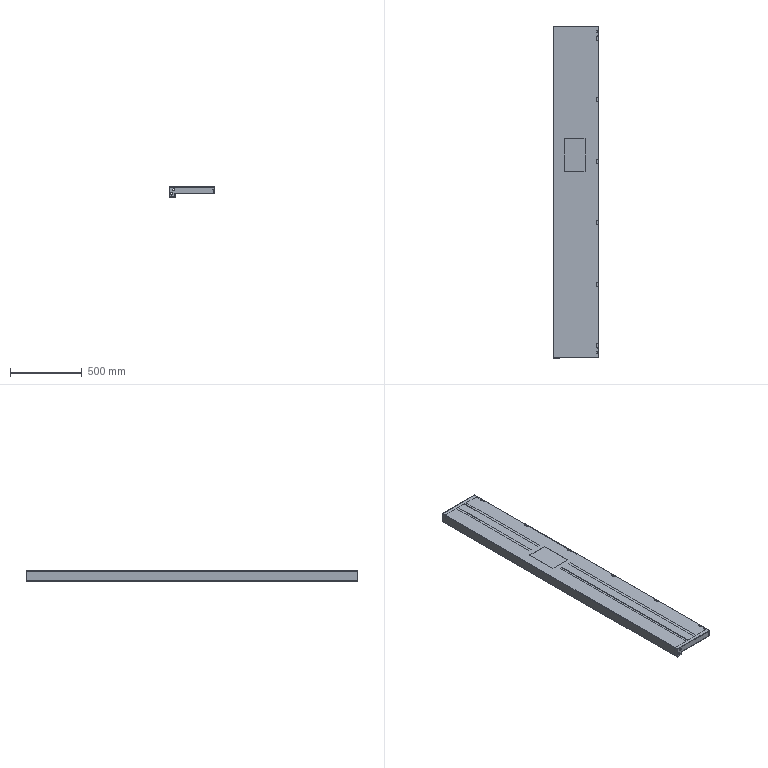Part | 6 solids | 384 faces | box 320 x 2316 x 70 mm | volume 2311859 mm3 | plane 246 | cylinder 138 | commonest cylinder face diameters 6 x28 6.2 x28 9 x18 11 x10 3.4 x9 2 x8